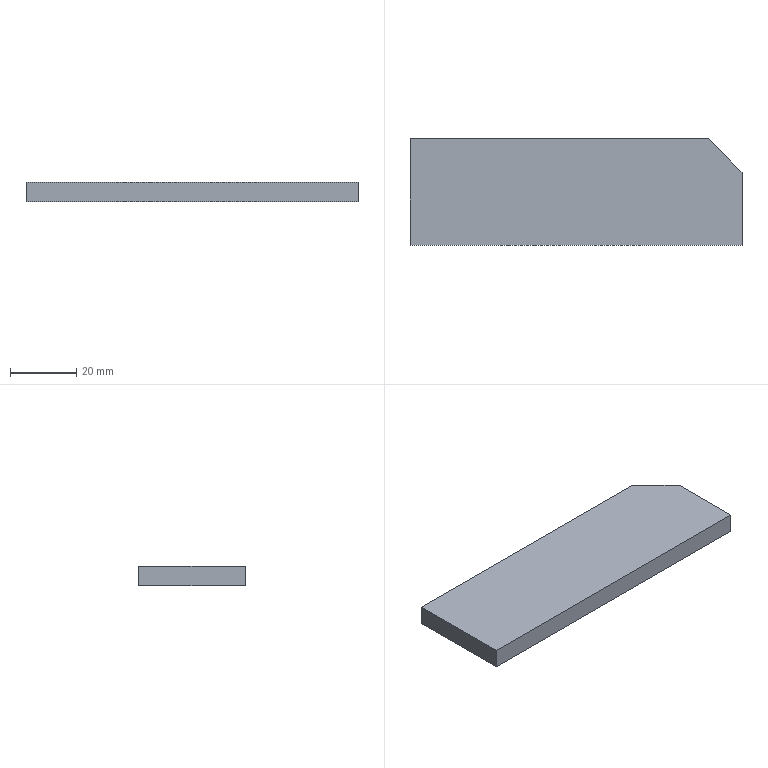Part | STEP file | [04] | 1 solid | 7 faces | box 100 x 32 x 6 mm | volume 18900 mm3 | plane 7
STEP:
#1=CARTESIAN_POINT('',(100.,22.,6.));
#2=VERTEX_POINT('',#1);
#3=CARTESIAN_POINT('',(100.,0.,6.));
#4=VERTEX_POINT('',#3);
#5=CARTESIAN_POINT('',(100.,16.,6.));
#6=DIRECTION('',(0.,-1.,0.));
#7=VECTOR('',#6,1000.);
#8=LINE('',#5,#7);
#9=EDGE_CURVE('',#2,#4,#8,.T.);
#10=ORIENTED_EDGE('',*,*,#9,.F.);
#11=CARTESIAN_POINT('',(90.,32.,6.));
#12=VERTEX_POINT('',#11);
#13=CARTESIAN_POINT('',(78.,44.,6.));
#14=DIRECTION('',(-0.7071,0.7071,0.));
#15=VECTOR('',#14,1000.);
#16=LINE('',#13,#15);
#17=EDGE_CURVE('',#2,#12,#16,.T.);
#18=ORIENTED_EDGE('',*,*,#17,.T.);
#19=CARTESIAN_POINT('',(0.,32.,6.));
#20=VERTEX_POINT('',#19);
#21=CARTESIAN_POINT('',(50.,32.,6.));
#22=DIRECTION('',(1.,0.,0.));
#23=VECTOR('',#22,1000.);
#24=LINE('',#21,#23);
#25=EDGE_CURVE('',#20,#12,#24,.T.);
#26=ORIENTED_EDGE('',*,*,#25,.F.);
#27=CARTESIAN_POINT('',(0.,0.,6.));
#28=VERTEX_POINT('',#27);
#29=CARTESIAN_POINT('',(0.,16.,6.));
#30=DIRECTION('',(0.,1.,0.));
#31=VECTOR('',#30,1000.);
#32=LINE('',#29,#31);
#33=EDGE_CURVE('',#28,#20,#32,.T.);
#34=ORIENTED_EDGE('',*,*,#33,.F.);
#35=CARTESIAN_POINT('',(50.,0.,6.));
#36=DIRECTION('',(-1.,0.,0.));
#37=VECTOR('',#36,1000.);
#38=LINE('',#35,#37);
#39=EDGE_CURVE('',#4,#28,#38,.T.);
#40=ORIENTED_EDGE('',*,*,#39,.F.);
#41=EDGE_LOOP('',(#10,#18,#26,#34,#40));
#42=FACE_OUTER_BOUND('',#41,.T.);
#43=CARTESIAN_POINT('',(50.,16.,6.));
#44=DIRECTION('',(0.,0.,1.));
#45=DIRECTION('',(1.,0.,0.));
#46=AXIS2_PLACEMENT_3D('',#43,#44,#45);
#47=PLANE('',#46);
#48=ADVANCED_FACE('',(#42),#47,.T.);
#49=CARTESIAN_POINT('',(100.,0.,0.));
#50=VERTEX_POINT('',#49);
#51=CARTESIAN_POINT('',(100.,0.,0.));
#52=DIRECTION('',(0.,0.,1.));
#53=VECTOR('',#52,1000.);
#54=LINE('',#51,#53);
#55=EDGE_CURVE('',#50,#4,#54,.T.);
#56=ORIENTED_EDGE('',*,*,#55,.T.);
#57=ORIENTED_EDGE('',*,*,#39,.T.);
#58=CARTESIAN_POINT('',(0.,0.,0.));
#59=VERTEX_POINT('',#58);
#60=CARTESIAN_POINT('',(0.,0.,0.));
#61=DIRECTION('',(0.,0.,1.));
#62=VECTOR('',#61,1000.);
#63=LINE('',#60,#62);
#64=EDGE_CURVE('',#59,#28,#63,.T.);
#65=ORIENTED_EDGE('',*,*,#64,.F.);
#66=CARTESIAN_POINT('',(50.,0.,0.));
#67=DIRECTION('',(1.,0.,0.));
#68=VECTOR('',#67,1000.);
#69=LINE('',#66,#68);
#70=EDGE_CURVE('',#59,#50,#69,.T.);
#71=ORIENTED_EDGE('',*,*,#70,.T.);
#72=EDGE_LOOP('',(#56,#57,#65,#71));
#73=FACE_OUTER_BOUND('',#72,.T.);
#74=CARTESIAN_POINT('',(50.,0.,0.));
#75=DIRECTION('',(0.,-1.,0.));
#76=DIRECTION('',(0.,0.,-1.));
#77=AXIS2_PLACEMENT_3D('',#74,#75,#76);
#78=PLANE('',#77);
#79=ADVANCED_FACE('',(#73),#78,.T.);
#80=ORIENTED_EDGE('',*,*,#64,.T.);
#81=ORIENTED_EDGE('',*,*,#33,.T.);
#82=CARTESIAN_POINT('',(0.,32.,0.));
#83=VERTEX_POINT('',#82);
#84=CARTESIAN_POINT('',(0.,32.,0.));
#85=DIRECTION('',(0.,0.,1.));
#86=VECTOR('',#85,1000.);
#87=LINE('',#84,#86);
#88=EDGE_CURVE('',#83,#20,#87,.T.);
#89=ORIENTED_EDGE('',*,*,#88,.F.);
#90=CARTESIAN_POINT('',(0.,16.,0.));
#91=DIRECTION('',(0.,-1.,0.));
#92=VECTOR('',#91,1000.);
#93=LINE('',#90,#92);
#94=EDGE_CURVE('',#83,#59,#93,.T.);
#95=ORIENTED_EDGE('',*,*,#94,.T.);
#96=EDGE_LOOP('',(#80,#81,#89,#95));
#97=FACE_OUTER_BOUND('',#96,.T.);
#98=CARTESIAN_POINT('',(0.,16.,0.));
#99=DIRECTION('',(-1.,0.,0.));
#100=DIRECTION('',(0.,0.,1.));
#101=AXIS2_PLACEMENT_3D('',#98,#99,#100);
#102=PLANE('',#101);
#103=ADVANCED_FACE('',(#97),#102,.T.);
#104=ORIENTED_EDGE('',*,*,#25,.T.);
#105=CARTESIAN_POINT('',(90.,32.,0.));
#106=VERTEX_POINT('',#105);
#107=CARTESIAN_POINT('',(90.,32.,0.));
#108=DIRECTION('',(0.,0.,-1.));
#109=VECTOR('',#108,1000.);
#110=LINE('',#107,#109);
#111=EDGE_CURVE('',#12,#106,#110,.T.);
#112=ORIENTED_EDGE('',*,*,#111,.T.);
#113=CARTESIAN_POINT('',(50.,32.,0.));
#114=DIRECTION('',(-1.,0.,0.));
#115=VECTOR('',#114,1000.);
#116=LINE('',#113,#115);
#117=EDGE_CURVE('',#106,#83,#116,.T.);
#118=ORIENTED_EDGE('',*,*,#117,.T.);
#119=ORIENTED_EDGE('',*,*,#88,.T.);
#120=EDGE_LOOP('',(#104,#112,#118,#119));
#121=FACE_OUTER_BOUND('',#120,.T.);
#122=CARTESIAN_POINT('',(50.,32.,0.));
#123=DIRECTION('',(0.,1.,0.));
#124=DIRECTION('',(0.,0.,1.));
#125=AXIS2_PLACEMENT_3D('',#122,#123,#124);
#126=PLANE('',#125);
#127=ADVANCED_FACE('',(#121),#126,.T.);
#128=ORIENTED_EDGE('',*,*,#117,.F.);
#129=CARTESIAN_POINT('',(100.,22.,0.));
#130=VERTEX_POINT('',#129);
#131=CARTESIAN_POINT('',(78.,44.,0.));
#132=DIRECTION('',(0.7071,-0.7071,0.));
#133=VECTOR('',#132,1000.);
#134=LINE('',#131,#133);
#135=EDGE_CURVE('',#106,#130,#134,.T.);
#136=ORIENTED_EDGE('',*,*,#135,.T.);
#137=CARTESIAN_POINT('',(100.,16.,0.));
#138=DIRECTION('',(0.,1.,0.));
#139=VECTOR('',#138,1000.);
#140=LINE('',#137,#139);
#141=EDGE_CURVE('',#50,#130,#140,.T.);
#142=ORIENTED_EDGE('',*,*,#141,.F.);
#143=ORIENTED_EDGE('',*,*,#70,.F.);
#144=ORIENTED_EDGE('',*,*,#94,.F.);
#145=EDGE_LOOP('',(#128,#136,#142,#143,#144));
#146=FACE_OUTER_BOUND('',#145,.T.);
#147=CARTESIAN_POINT('',(50.,16.,0.));
#148=DIRECTION('',(0.,0.,-1.));
#149=DIRECTION('',(-1.,0.,0.));
#150=AXIS2_PLACEMENT_3D('',#147,#148,#149);
#151=PLANE('',#150);
#152=ADVANCED_FACE('',(#146),#151,.T.);
#153=ORIENTED_EDGE('',*,*,#141,.T.);
#154=CARTESIAN_POINT('',(100.,22.,0.));
#155=DIRECTION('',(0.,0.,1.));
#156=VECTOR('',#155,1000.);
#157=LINE('',#154,#156);
#158=EDGE_CURVE('',#130,#2,#157,.T.);
#159=ORIENTED_EDGE('',*,*,#158,.T.);
#160=ORIENTED_EDGE('',*,*,#9,.T.);
#161=ORIENTED_EDGE('',*,*,#55,.F.);
#162=EDGE_LOOP('',(#153,#159,#160,#161));
#163=FACE_OUTER_BOUND('',#162,.T.);
#164=CARTESIAN_POINT('',(100.,16.,0.));
#165=DIRECTION('',(1.,0.,0.));
#166=DIRECTION('',(0.,0.,-1.));
#167=AXIS2_PLACEMENT_3D('',#164,#165,#166);
#168=PLANE('',#167);
#169=ADVANCED_FACE('',(#163),#168,.T.);
#170=ORIENTED_EDGE('',*,*,#135,.F.);
#171=ORIENTED_EDGE('',*,*,#111,.F.);
#172=ORIENTED_EDGE('',*,*,#17,.F.);
#173=ORIENTED_EDGE('',*,*,#158,.F.);
#174=EDGE_LOOP('',(#170,#171,#172,#173));
#175=FACE_OUTER_BOUND('',#174,.T.);
#176=CARTESIAN_POINT('',(100.,22.,0.));
#177=DIRECTION('',(-0.7071,-0.7071,0.));
#178=DIRECTION('',(0.,0.,1.));
#179=AXIS2_PLACEMENT_3D('',#176,#177,#178);
#180=PLANE('',#179);
#181=ADVANCED_FACE('',(#175),#180,.F.);
#182=CLOSED_SHELL('',(#48,#79,#103,#127,#152,#169,#181));
#183=MANIFOLD_SOLID_BREP('',#182);
#184=CARTESIAN_POINT('',(0.,0.,0.));
#185=DIRECTION('',(0.,0.,1.));
#186=DIRECTION('',(1.,0.,0.));
#187=AXIS2_PLACEMENT_3D('',#184,#185,#186);
#188=(LENGTH_UNIT()NAMED_UNIT(*)SI_UNIT(.MILLI.,.METRE.));
#189=UNCERTAINTY_MEASURE_WITH_UNIT(LENGTH_MEASURE(0.00001),#188,'','');
#190=(NAMED_UNIT(*)PLANE_ANGLE_UNIT()SI_UNIT($,.RADIAN.));
#191=(NAMED_UNIT(*)SI_UNIT($,.STERADIAN.)SOLID_ANGLE_UNIT());
#192=(GEOMETRIC_REPRESENTATION_CONTEXT(3)GLOBAL_UNCERTAINTY_ASSIGNED_CONTEXT((#189))GLOBAL_UNIT_ASSIGNED_CONTEXT((#188,#190,#191))REPRESENTATION_CONTEXT('',''));
#193=ADVANCED_BREP_SHAPE_REPRESENTATION('',(#183,#187),#192);